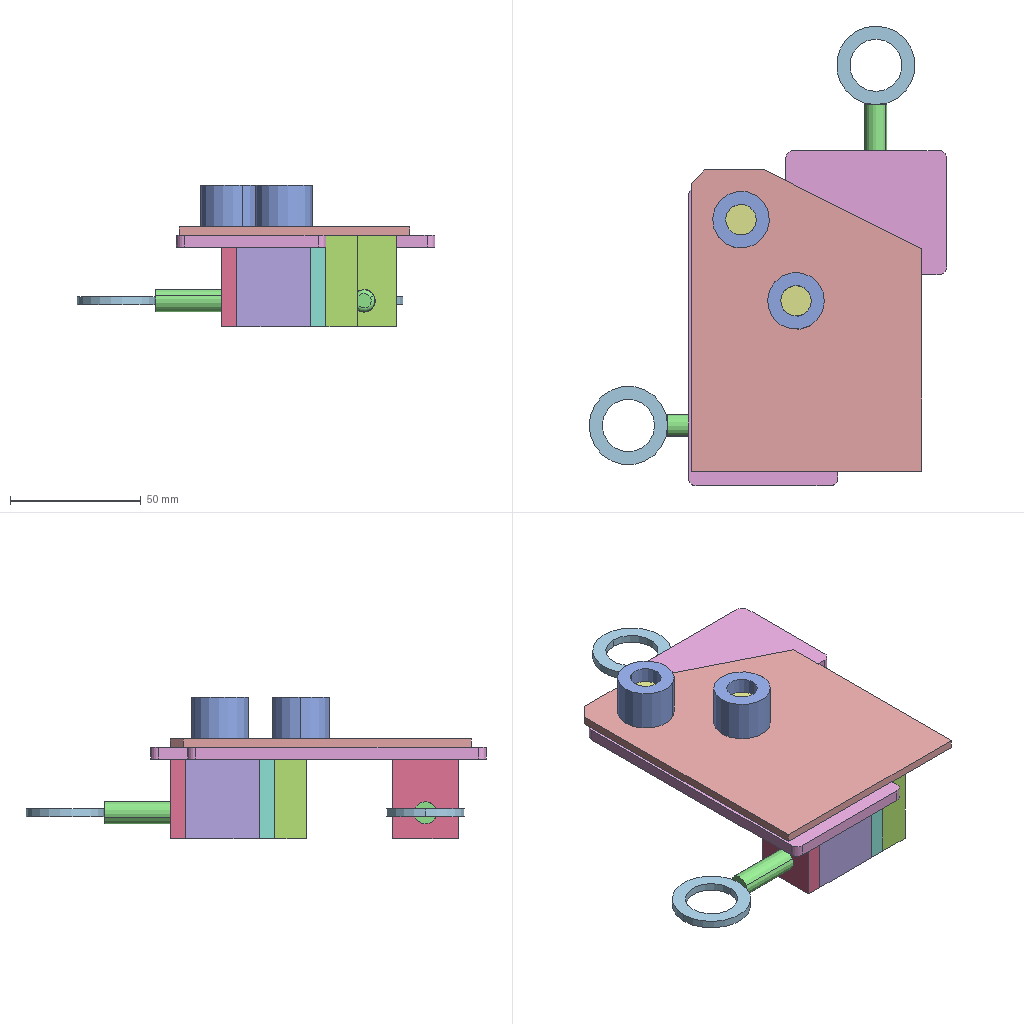Assembly | SolidWorks | 11 different items | 22 placed | box 137 x 176 x 54 mm
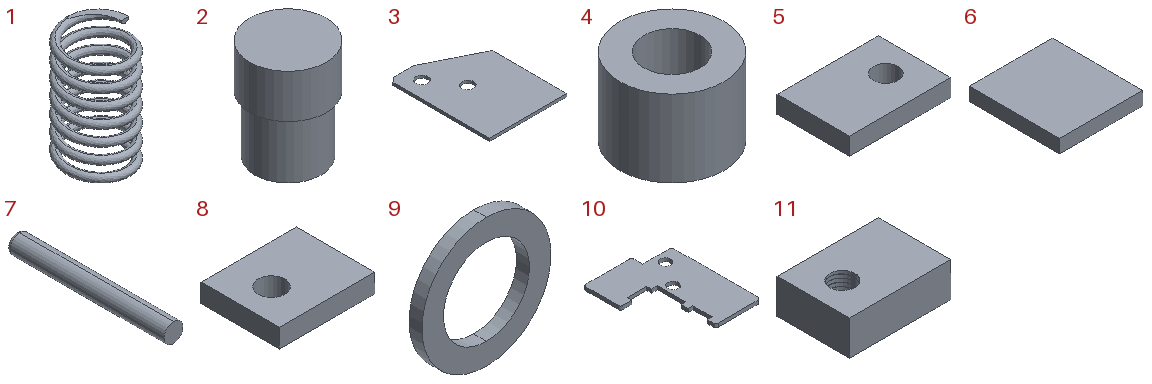Parts list (item | quantity | size | volume | features):
1 | x2 | 17 x 17 x 28 mm | 1021 mm3 | features Split 2, Helix 1, Sweep 1
2 | x2 | 13.5 x 13.5 x 17.7 mm | 2177 mm3 | features ICE 2, Extrusion 1
3 | x1 | 88 x 115 x 3.2 mm | 28548 mm3 | features FlatPattern 1, SMBaseFlange 1, SheetMetal 1
4 | x2 | 21.7 x 21.7 x 16 mm | 4197 mm3 | features Extrusion 1
5 | x2 | 35 x 25 x 6 mm | 4910 mm3 | features FlatPattern 1, SMBaseFlange 1, SheetMetal 1
6 | x4 | 28 x 30.5 x 4.5 mm | 3843 mm3 | features FlatPattern 1, SMBaseFlange 1, SheetMetal 1
7 | x2 | 8.5 x 70 x 8.5 mm | 3960 mm3 | features Extrusion 1, Fillet 1
8 | x2 | 30.5 x 25 x 6 mm | 4235 mm3 | features Extrusion 1
9 | x2 | 30 x 3 x 30 mm | 1178 mm3 | features Extrusion 1
10 | x1 | 98.706 x 128.023 x 4.5 mm | 35781 mm3 | features FlatPattern 1, SMBaseFlange 1, SheetMetal 1
11 | x2 | 35 x 25 x 12 mm | 9818 mm3 | features Extrusion 1, Helix 1, SweepCut 1
Mates (type | each side: item.copy, entity, surface, feature):
Concentric | 3.1 edge | 4.1 edge
Coincident | 3.1 face plane Base-Flange1 | 4.1 face plane Boss-Extrude1
Concentric | 3.1 edge | 4.2 edge
Coincident | 3.1 face plane Base-Flange1 | 4.2 face plane Boss-Extrude1
Parallel | 3.1 face plane Base-Flange1 | 11.1 face plane Boss-Extrude1
Coincident | 3.1 face plane Base-Flange1 | 11.1 face plane Boss-Extrude1
DistanceDim | 11.1 face plane Boss-Extrude1 | 3.1 face plane Base-Flange1
Coincident | 3.1 face plane Base-Flange1 | 11.2 face plane Boss-Extrude1
DistanceDim | 11.2 face plane Boss-Extrude1 | 3.1 face plane Base-Flange1 | 2 times
Parallel | 3.1 face plane Base-Flange1 | 11.2 face plane Boss-Extrude1
DistanceDim | 3.1 face plane Base-Flange1 | 11.1 face plane Boss-Extrude1
Parallel | 3.1 face plane Base-Flange1 | 10.1 face plane Base-Flange1 | 2 times
Concentric | 3.1 edge | 10.1 edge
Coincident | 3.1 face plane Base-Flange1 | 10.1 face plane Base-Flange1
Coincident | 3.1 face plane Base-Flange1 | 5.1 face plane Base-Flange1
Coincident | 11.2 face plane Boss-Extrude1 | 5.1 face plane Base-Flange1
Coincident | 10.1 face plane Base-Flange1 | 5.1 face plane Base-Flange1
Coincident | 3.1 face plane Base-Flange1 | 5.2 face plane Base-Flange1
Coincident | 10.1 face plane Base-Flange1 | 5.2 face plane Base-Flange1
Coincident | 11.1 face plane Boss-Extrude1 | 5.2 face plane Base-Flange1
Concentric | 5.2 edge | 1.1 select_type:24
Coincident | 5.2 face plane Base-Flange1 | 1.1 face plane Split2
Coincident | 5.1 face plane Base-Flange1 | 1.2 face plane Split2
Concentric | 5.1 edge | 1.2 select_type:24
Coincident | 5.2 face plane Base-Flange1 | 6.1 face plane Base-Flange1 | 3 times
Concentric | 5.2 edge | 7.1 edge
DistanceDim | 7.1 face plane Boss-Extrude1 | 5.2 face plane Base-Flange1
Concentric | 5.1 edge | 7.2 edge
DistanceDim | 7.2 face plane Boss-Extrude1 | 5.1 face plane Base-Flange1
Coincident | 1.2 face plane Split1 | 8.1 face plane Boss-Extrude1
Concentric | 1.2 select_type:24 | 8.1 edge
Coincident | 5.1 face plane Base-Flange1 | 8.1 face plane Boss-Extrude1
Concentric | 1.1 select_type:24 | 8.2 edge
Coincident | 1.1 face plane Split1 | 8.2 face plane Boss-Extrude1
Coincident | 5.2 face plane Base-Flange1 | 8.2 face plane Boss-Extrude1
Coincident | 5.2 face plane Base-Flange1 | 6.2 face plane Base-Flange1 | 2 times
Coincident | 6.1 face plane Base-Flange1 | 6.2 face plane Base-Flange1
Coincident | 8.1 face plane Boss-Extrude1 | 6.3 face plane Base-Flange1
Coincident | 10.1 face plane Base-Flange1 | 6.3 face plane Base-Flange1
Coincident | 5.1 face plane Base-Flange1 | 6.3 face plane Base-Flange1 | 2 times
Coincident | 8.1 face plane Boss-Extrude1 | 6.4 face plane Base-Flange1 | 2 times
Coincident | 6.3 face plane Base-Flange1 | 6.4 face plane Base-Flange1
Concentric | 7.1 edge | 9.1 select_type:24
Coincident | 7.1 face plane Boss-Extrude1 | 9.1 select_type:24
Parallel | 10.1 face plane Base-Flange1 | 9.1 face plane Boss-Extrude1
Coincident | 7.2 face plane Boss-Extrude1 | 9.2 select_type:24
Concentric | 7.2 edge | 9.2 select_type:24
Parallel | 10.1 face plane Base-Flange1 | 9.2 face plane Boss-Extrude1
Coincident | 10.1 edge | 2.1 edge